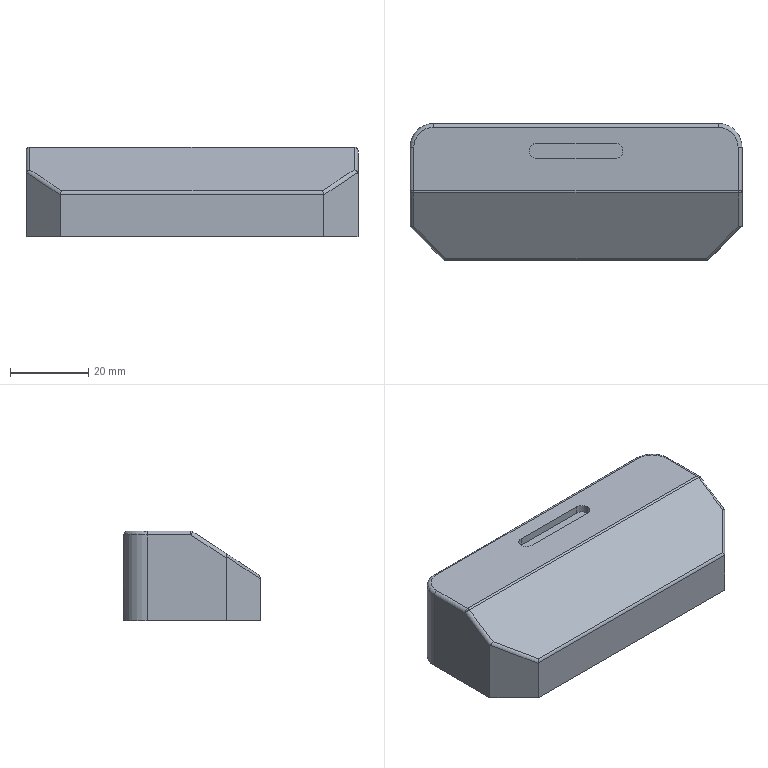Part | NX | features BREP 1 | 1 solid | 65 faces | box 85 x 35 x 23 mm | volume 24223 mm3 | plane 41 | cylinder 20 | sphere 2 | torus 2 | commonest cylinder face diameters 2 x9 8.5 x4 4 x3 12 x2 14.5 x2